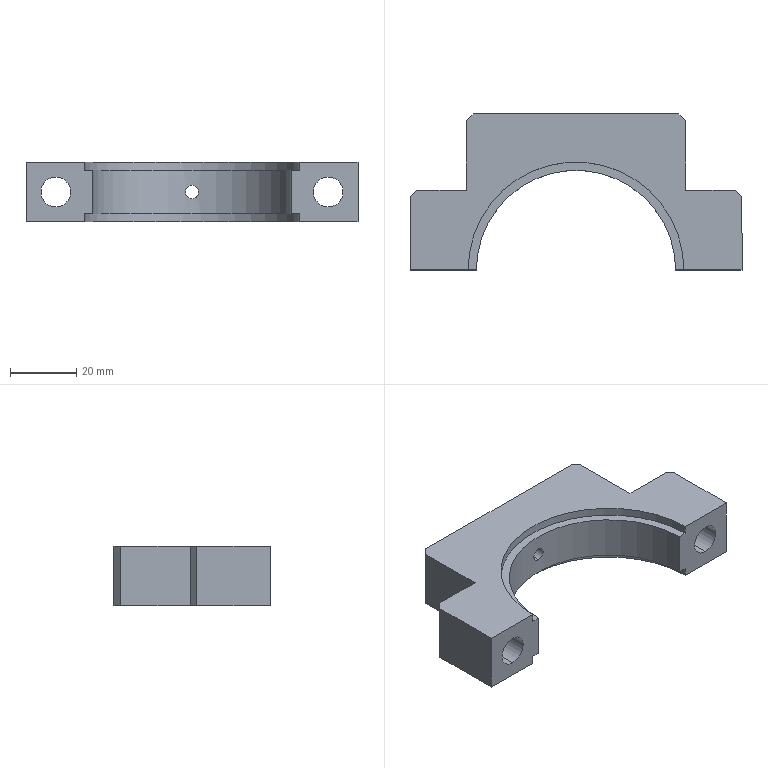Part | SolidWorks | features HoleWzd 3, ICE 2, Chamfer 1, Extrusion 1 | 1 solid | 30 faces | box 100 x 47 x 18 mm | volume 40091 mm3 | plane 17 | cylinder 11 | cone 2 | commonest cylinder face diameters 9 x4 4 x2 7 x2 65 x2 60 x1
STEP:
#1=CARTESIAN_POINT('',(0.,30.,7.));
#2=VERTEX_POINT('',#1);
#3=CARTESIAN_POINT('',(0.,30.,11.));
#4=VERTEX_POINT('',#3);
#5=CARTESIAN_POINT('',(0.,30.,7.));
#6=CARTESIAN_POINT('',(-0.261,30.,7.));
#7=CARTESIAN_POINT('',(-0.5242,29.996,7.052));
#8=CARTESIAN_POINT('',(-1.006,29.984,7.252));
#9=CARTESIAN_POINT('',(-1.229,29.975,7.401));
#10=CARTESIAN_POINT('',(-1.505,29.962,7.677));
#11=CARTESIAN_POINT('',(-1.59,29.958,7.78));
#12=CARTESIAN_POINT('',(-1.735,29.95,7.997));
#13=CARTESIAN_POINT('',(-1.797,29.946,8.112));
#14=CARTESIAN_POINT('',(-1.897,29.94,8.354));
#15=CARTESIAN_POINT('',(-1.936,29.937,8.481));
#16=CARTESIAN_POINT('',(-1.987,29.934,8.737));
#17=CARTESIAN_POINT('',(-2.,29.933,8.866));
#18=CARTESIAN_POINT('',(-2.,29.933,9.13));
#19=CARTESIAN_POINT('',(-1.987,29.934,9.261));
#20=CARTESIAN_POINT('',(-1.937,29.937,9.516));
#21=CARTESIAN_POINT('',(-1.898,29.94,9.643));
#22=CARTESIAN_POINT('',(-1.798,29.946,9.886));
#23=CARTESIAN_POINT('',(-1.737,29.95,10.001));
#24=CARTESIAN_POINT('',(-1.592,29.958,10.218));
#25=CARTESIAN_POINT('',(-1.507,29.962,10.321));
#26=CARTESIAN_POINT('',(-1.323,29.971,10.506));
#27=CARTESIAN_POINT('',(-1.222,29.975,10.588));
#28=CARTESIAN_POINT('',(-1.004,29.983,10.735));
#29=CARTESIAN_POINT('',(-0.8877,29.987,10.797));
#30=CARTESIAN_POINT('',(-0.5269,29.996,10.947));
#31=CARTESIAN_POINT('',(-0.2643,30.,11.));
#32=CARTESIAN_POINT('',(0.,30.,11.));
#33=B_SPLINE_CURVE_WITH_KNOTS('',3,(#5,#6,#7,#8,#9,#10,#11,#12,#13,#14,#15,#16,#17,#18,#19,#20,#21,#22,#23,#24,#25,#26,#27,#28,#29,#30,#31,#32),.UNSPECIFIED.,.F.,.F.,(4,2,2,2,2,2,2,2,2,2,2,2,2,4),(0.006255,0.007036,0.007818,0.008209,0.0086,0.00899,0.009381,0.009772,0.01016,0.01055,0.01094,0.01134,0.01173,0.01251),.UNSPECIFIED.);
#34=EDGE_CURVE('',#2,#4,#33,.T.);
#35=ORIENTED_EDGE('',*,*,#34,.F.);
#36=CARTESIAN_POINT('',(0.,33.099,7.));
#37=VERTEX_POINT('',#36);
#38=CARTESIAN_POINT('',(0.,47.,7.));
#39=DIRECTION('',(0.,1.,0.));
#40=VECTOR('',#39,1000.);
#41=LINE('',#38,#40);
#42=EDGE_CURVE('',#2,#37,#41,.T.);
#43=ORIENTED_EDGE('',*,*,#42,.T.);
#44=CARTESIAN_POINT('',(0.,33.099,11.));
#45=VERTEX_POINT('',#44);
#46=CARTESIAN_POINT('',(0.,33.099,9.));
#47=DIRECTION('',(0.,-1.,0.));
#48=DIRECTION('',(0.,0.,1.));
#49=AXIS2_PLACEMENT_3D('',#46,#47,#48);
#50=CIRCLE('',#49,2.);
#51=EDGE_CURVE('',#45,#37,#50,.T.);
#52=ORIENTED_EDGE('',*,*,#51,.F.);
#53=CARTESIAN_POINT('',(0.,47.,11.));
#54=DIRECTION('',(0.,1.,0.));
#55=VECTOR('',#54,1000.);
#56=LINE('',#53,#55);
#57=EDGE_CURVE('',#4,#45,#56,.T.);
#58=ORIENTED_EDGE('',*,*,#57,.F.);
#59=EDGE_LOOP('',(#35,#43,#52,#58));
#60=FACE_OUTER_BOUND('',#59,.T.);
#61=CARTESIAN_POINT('',(0.,47.,9.));
#62=DIRECTION('',(0.,1.,0.));
#63=DIRECTION('',(0.,0.,1.));
#64=AXIS2_PLACEMENT_3D('',#61,#62,#63);
#65=CYLINDRICAL_SURFACE('',#64,2.);
#66=ADVANCED_FACE('',(#60),#65,.F.);
#67=CARTESIAN_POINT('',(-41.,0.,4.5));
#68=VERTEX_POINT('',#67);
#69=CARTESIAN_POINT('',(-41.,0.,13.5));
#70=VERTEX_POINT('',#69);
#71=CARTESIAN_POINT('',(-41.,0.,9.));
#72=DIRECTION('',(0.,1.,0.));
#73=DIRECTION('',(0.,0.,1.));
#74=AXIS2_PLACEMENT_3D('',#71,#72,#73);
#75=CIRCLE('',#74,4.5);
#76=EDGE_CURVE('',#68,#70,#75,.T.);
#77=ORIENTED_EDGE('',*,*,#76,.F.);
#78=CARTESIAN_POINT('',(-41.,24.,4.5));
#79=VERTEX_POINT('',#78);
#80=CARTESIAN_POINT('',(-41.,24.,4.5));
#81=DIRECTION('',(0.,1.,0.));
#82=VECTOR('',#81,1000.);
#83=LINE('',#80,#82);
#84=EDGE_CURVE('',#68,#79,#83,.T.);
#85=ORIENTED_EDGE('',*,*,#84,.T.);
#86=CARTESIAN_POINT('',(-41.,24.,13.5));
#87=VERTEX_POINT('',#86);
#88=CARTESIAN_POINT('',(-41.,24.,9.));
#89=DIRECTION('',(0.,1.,0.));
#90=DIRECTION('',(0.,0.,1.));
#91=AXIS2_PLACEMENT_3D('',#88,#89,#90);
#92=CIRCLE('',#91,4.5);
#93=EDGE_CURVE('',#79,#87,#92,.T.);
#94=ORIENTED_EDGE('',*,*,#93,.T.);
#95=CARTESIAN_POINT('',(-41.,24.,13.5));
#96=DIRECTION('',(0.,1.,0.));
#97=VECTOR('',#96,1000.);
#98=LINE('',#95,#97);
#99=EDGE_CURVE('',#70,#87,#98,.T.);
#100=ORIENTED_EDGE('',*,*,#99,.F.);
#101=EDGE_LOOP('',(#77,#85,#94,#100));
#102=FACE_OUTER_BOUND('',#101,.T.);
#103=CARTESIAN_POINT('',(-41.,24.,9.));
#104=DIRECTION('',(0.,1.,0.));
#105=DIRECTION('',(0.,0.,1.));
#106=AXIS2_PLACEMENT_3D('',#103,#104,#105);
#107=CYLINDRICAL_SURFACE('',#106,4.5);
#108=ADVANCED_FACE('',(#102),#107,.F.);
#109=CARTESIAN_POINT('',(41.,0.,4.5));
#110=VERTEX_POINT('',#109);
#111=CARTESIAN_POINT('',(41.,0.,13.5));
#112=VERTEX_POINT('',#111);
#113=CARTESIAN_POINT('',(41.,0.,9.));
#114=DIRECTION('',(0.,1.,0.));
#115=DIRECTION('',(0.,0.,1.));
#116=AXIS2_PLACEMENT_3D('',#113,#114,#115);
#117=CIRCLE('',#116,4.5);
#118=EDGE_CURVE('',#110,#112,#117,.T.);
#119=ORIENTED_EDGE('',*,*,#118,.F.);
#120=CARTESIAN_POINT('',(41.,24.,4.5));
#121=VERTEX_POINT('',#120);
#122=CARTESIAN_POINT('',(41.,24.,4.5));
#123=DIRECTION('',(0.,1.,0.));
#124=VECTOR('',#123,1000.);
#125=LINE('',#122,#124);
#126=EDGE_CURVE('',#110,#121,#125,.T.);
#127=ORIENTED_EDGE('',*,*,#126,.T.);
#128=CARTESIAN_POINT('',(41.,24.,13.5));
#129=VERTEX_POINT('',#128);
#130=CARTESIAN_POINT('',(41.,24.,9.));
#131=DIRECTION('',(0.,1.,0.));
#132=DIRECTION('',(0.,0.,1.));
#133=AXIS2_PLACEMENT_3D('',#130,#131,#132);
#134=CIRCLE('',#133,4.5);
#135=EDGE_CURVE('',#121,#129,#134,.T.);
#136=ORIENTED_EDGE('',*,*,#135,.T.);
#137=CARTESIAN_POINT('',(41.,24.,13.5));
#138=DIRECTION('',(0.,1.,0.));
#139=VECTOR('',#138,1000.);
#140=LINE('',#137,#139);
#141=EDGE_CURVE('',#112,#129,#140,.T.);
#142=ORIENTED_EDGE('',*,*,#141,.F.);
#143=EDGE_LOOP('',(#119,#127,#136,#142));
#144=FACE_OUTER_BOUND('',#143,.T.);
#145=CARTESIAN_POINT('',(41.,24.,9.));
#146=DIRECTION('',(0.,1.,0.));
#147=DIRECTION('',(0.,0.,1.));
#148=AXIS2_PLACEMENT_3D('',#145,#146,#147);
#149=CYLINDRICAL_SURFACE('',#148,4.5);
#150=ADVANCED_FACE('',(#144),#149,.F.);
#151=CARTESIAN_POINT('',(0.,34.,5.5));
#152=VERTEX_POINT('',#151);
#153=CARTESIAN_POINT('',(0.,34.,12.5));
#154=VERTEX_POINT('',#153);
#155=CARTESIAN_POINT('',(0.,34.,9.));
#156=DIRECTION('',(0.,1.,0.));
#157=DIRECTION('',(0.,0.,1.));
#158=AXIS2_PLACEMENT_3D('',#155,#156,#157);
#159=CIRCLE('',#158,3.5);
#160=EDGE_CURVE('',#152,#154,#159,.T.);
#161=ORIENTED_EDGE('',*,*,#160,.F.);
#162=CARTESIAN_POINT('',(0.,47.,5.5));
#163=VERTEX_POINT('',#162);
#164=CARTESIAN_POINT('',(0.,47.,5.5));
#165=DIRECTION('',(0.,1.,0.));
#166=VECTOR('',#165,1000.);
#167=LINE('',#164,#166);
#168=EDGE_CURVE('',#152,#163,#167,.T.);
#169=ORIENTED_EDGE('',*,*,#168,.T.);
#170=CARTESIAN_POINT('',(0.,47.,12.5));
#171=VERTEX_POINT('',#170);
#172=CARTESIAN_POINT('',(0.,47.,9.));
#173=DIRECTION('',(0.,1.,0.));
#174=DIRECTION('',(0.,0.,1.));
#175=AXIS2_PLACEMENT_3D('',#172,#173,#174);
#176=CIRCLE('',#175,3.5);
#177=EDGE_CURVE('',#163,#171,#176,.T.);
#178=ORIENTED_EDGE('',*,*,#177,.T.);
#179=CARTESIAN_POINT('',(0.,47.,12.5));
#180=DIRECTION('',(0.,1.,0.));
#181=VECTOR('',#180,1000.);
#182=LINE('',#179,#181);
#183=EDGE_CURVE('',#154,#171,#182,.T.);
#184=ORIENTED_EDGE('',*,*,#183,.F.);
#185=EDGE_LOOP('',(#161,#169,#178,#184));
#186=FACE_OUTER_BOUND('',#185,.T.);
#187=CARTESIAN_POINT('',(0.,47.,9.));
#188=DIRECTION('',(0.,1.,0.));
#189=DIRECTION('',(0.,0.,1.));
#190=AXIS2_PLACEMENT_3D('',#187,#188,#189);
#191=CYLINDRICAL_SURFACE('',#190,3.5);
#192=ADVANCED_FACE('',(#186),#191,.F.);
#193=ORIENTED_EDGE('',*,*,#51,.T.);
#194=CARTESIAN_POINT('',(0.,34.,5.5));
#195=DIRECTION('',(0.,0.515,-0.8572));
#196=VECTOR('',#195,1000.);
#197=LINE('',#194,#196);
#198=EDGE_CURVE('',#37,#152,#197,.T.);
#199=ORIENTED_EDGE('',*,*,#198,.T.);
#200=ORIENTED_EDGE('',*,*,#160,.T.);
#201=CARTESIAN_POINT('',(0.,34.,12.5));
#202=DIRECTION('',(0.,0.515,0.8572));
#203=VECTOR('',#202,1000.);
#204=LINE('',#201,#203);
#205=EDGE_CURVE('',#45,#154,#204,.T.);
#206=ORIENTED_EDGE('',*,*,#205,.F.);
#207=EDGE_LOOP('',(#193,#199,#200,#206));
#208=FACE_OUTER_BOUND('',#207,.T.);
#209=CARTESIAN_POINT('',(0.,34.,9.));
#210=DIRECTION('',(0.,1.,0.));
#211=DIRECTION('',(0.,0.,1.));
#212=AXIS2_PLACEMENT_3D('',#209,#210,#211);
#213=CONICAL_SURFACE('',#212,3.5,1.03);
#214=ADVANCED_FACE('',(#208),#213,.F.);
#215=CARTESIAN_POINT('',(0.,30.,11.));
#216=CARTESIAN_POINT('',(0.1322,30.,11.));
#217=CARTESIAN_POINT('',(0.2622,29.999,10.987));
#218=CARTESIAN_POINT('',(0.5178,29.996,10.936));
#219=CARTESIAN_POINT('',(0.6449,29.993,10.898));
#220=CARTESIAN_POINT('',(0.8871,29.987,10.797));
#221=CARTESIAN_POINT('',(1.002,29.983,10.736));
#222=CARTESIAN_POINT('',(1.219,29.975,10.591));
#223=CARTESIAN_POINT('',(1.322,29.971,10.506));
#224=CARTESIAN_POINT('',(1.599,29.958,10.229));
#225=CARTESIAN_POINT('',(1.748,29.949,10.006));
#226=CARTESIAN_POINT('',(1.947,29.937,9.525));
#227=CARTESIAN_POINT('',(2.,29.933,9.262));
#228=CARTESIAN_POINT('',(2.,29.933,8.87));
#229=CARTESIAN_POINT('',(1.987,29.934,8.738));
#230=CARTESIAN_POINT('',(1.936,29.937,8.481));
#231=CARTESIAN_POINT('',(1.898,29.94,8.356));
#232=CARTESIAN_POINT('',(1.798,29.946,8.114));
#233=CARTESIAN_POINT('',(1.735,29.95,7.997));
#234=CARTESIAN_POINT('',(1.591,29.958,7.78));
#235=CARTESIAN_POINT('',(1.508,29.962,7.679));
#236=CARTESIAN_POINT('',(1.321,29.971,7.493));
#237=CARTESIAN_POINT('',(1.22,29.975,7.41));
#238=CARTESIAN_POINT('',(1.003,29.983,7.265));
#239=CARTESIAN_POINT('',(0.8865,29.987,7.202));
#240=CARTESIAN_POINT('',(0.6442,29.993,7.102));
#241=CARTESIAN_POINT('',(0.5195,29.996,7.064));
#242=CARTESIAN_POINT('',(0.2631,29.999,7.013));
#243=CARTESIAN_POINT('',(0.1305,30.,7.));
#244=CARTESIAN_POINT('',(0.,30.,7.));
#245=B_SPLINE_CURVE_WITH_KNOTS('',3,(#215,#216,#217,#218,#219,#220,#221,#222,#223,#224,#225,#226,#227,#228,#229,#230,#231,#232,#233,#234,#235,#236,#237,#238,#239,#240,#241,#242,#243,#244),.UNSPECIFIED.,.F.,.F.,(4,2,2,2,2,2,2,2,2,2,2,2,2,2,4),(0.,0.0003909,0.0007818,0.001173,0.001564,0.002345,0.003127,0.003518,0.003909,0.0043,0.004691,0.005082,0.005473,0.005864,0.006255),.UNSPECIFIED.);
#246=EDGE_CURVE('',#4,#2,#245,.T.);
#247=ORIENTED_EDGE('',*,*,#246,.T.);
#248=ORIENTED_EDGE('',*,*,#34,.T.);
#249=EDGE_LOOP('',(#247,#248));
#250=FACE_BOUND('',#249,.T.);
#251=CARTESIAN_POINT('',(-30.,0.,15.5));
#252=VERTEX_POINT('',#251);
#253=CARTESIAN_POINT('',(30.,0.,15.5));
#254=VERTEX_POINT('',#253);
#255=CARTESIAN_POINT('',(0.,0.,15.5));
#256=DIRECTION('',(0.,0.,-1.));
#257=DIRECTION('',(1.,0.,0.));
#258=AXIS2_PLACEMENT_3D('',#255,#256,#257);
#259=CIRCLE('',#258,30.);
#260=EDGE_CURVE('',#252,#254,#259,.T.);
#261=ORIENTED_EDGE('',*,*,#260,.F.);
#262=CARTESIAN_POINT('',(-30.,0.,2.5));
#263=VERTEX_POINT('',#262);
#264=CARTESIAN_POINT('',(-30.,0.,18.));
#265=DIRECTION('',(0.,0.,-1.));
#266=VECTOR('',#265,1000.);
#267=LINE('',#264,#266);
#268=EDGE_CURVE('',#252,#263,#267,.T.);
#269=ORIENTED_EDGE('',*,*,#268,.T.);
#270=CARTESIAN_POINT('',(30.,0.,2.5));
#271=VERTEX_POINT('',#270);
#272=CARTESIAN_POINT('',(0.,0.,2.5));
#273=DIRECTION('',(0.,0.,1.));
#274=DIRECTION('',(-1.,0.,0.));
#275=AXIS2_PLACEMENT_3D('',#272,#273,#274);
#276=CIRCLE('',#275,30.);
#277=EDGE_CURVE('',#271,#263,#276,.T.);
#278=ORIENTED_EDGE('',*,*,#277,.F.);
#279=CARTESIAN_POINT('',(30.,0.,18.));
#280=DIRECTION('',(0.,0.,-1.));
#281=VECTOR('',#280,1000.);
#282=LINE('',#279,#281);
#283=EDGE_CURVE('',#254,#271,#282,.T.);
#284=ORIENTED_EDGE('',*,*,#283,.F.);
#285=EDGE_LOOP('',(#261,#269,#278,#284));
#286=FACE_OUTER_BOUND('',#285,.T.);
#287=CARTESIAN_POINT('',(0.,0.,18.));
#288=DIRECTION('',(0.,0.,-1.));
#289=DIRECTION('',(-1.,0.,0.));
#290=AXIS2_PLACEMENT_3D('',#287,#288,#289);
#291=CYLINDRICAL_SURFACE('',#290,30.);
#292=ADVANCED_FACE('',(#250,#286),#291,.F.);
#293=CARTESIAN_POINT('',(-50.,22.,18.));
#294=VERTEX_POINT('',#293);
#295=CARTESIAN_POINT('',(-50.,0.,18.));
#296=VERTEX_POINT('',#295);
#297=CARTESIAN_POINT('',(-50.,0.,18.));
#298=DIRECTION('',(0.,-1.,0.));
#299=VECTOR('',#298,1000.);
#300=LINE('',#297,#299);
#301=EDGE_CURVE('',#294,#296,#300,.T.);
#302=ORIENTED_EDGE('',*,*,#301,.F.);
#303=CARTESIAN_POINT('',(-50.,22.,0.));
#304=VERTEX_POINT('',#303);
#305=CARTESIAN_POINT('',(-50.,22.,18.));
#306=DIRECTION('',(0.,0.,-1.));
#307=VECTOR('',#306,1000.);
#308=LINE('',#305,#307);
#309=EDGE_CURVE('',#294,#304,#308,.T.);
#310=ORIENTED_EDGE('',*,*,#309,.T.);
#311=CARTESIAN_POINT('',(-50.,0.,0.));
#312=VERTEX_POINT('',#311);
#313=CARTESIAN_POINT('',(-50.,0.,0.));
#314=DIRECTION('',(0.,-1.,0.));
#315=VECTOR('',#314,1000.);
#316=LINE('',#313,#315);
#317=EDGE_CURVE('',#304,#312,#316,.T.);
#318=ORIENTED_EDGE('',*,*,#317,.T.);
#319=CARTESIAN_POINT('',(-50.,0.,18.));
#320=DIRECTION('',(0.,0.,-1.));
#321=VECTOR('',#320,1000.);
#322=LINE('',#319,#321);
#323=EDGE_CURVE('',#296,#312,#322,.T.);
#324=ORIENTED_EDGE('',*,*,#323,.F.);
#325=EDGE_LOOP('',(#302,#310,#318,#324));
#326=FACE_OUTER_BOUND('',#325,.T.);
#327=CARTESIAN_POINT('',(-50.,0.,18.));
#328=DIRECTION('',(1.,0.,0.));
#329=DIRECTION('',(0.,0.,-1.));
#330=AXIS2_PLACEMENT_3D('',#327,#328,#329);
#331=PLANE('',#330);
#332=ADVANCED_FACE('',(#326),#331,.F.);
#333=CARTESIAN_POINT('',(-41.,0.,9.));
#334=DIRECTION('',(0.,1.,0.));
#335=DIRECTION('',(0.,0.,1.));
#336=AXIS2_PLACEMENT_3D('',#333,#334,#335);
#337=CIRCLE('',#336,4.5);
#338=EDGE_CURVE('',#70,#68,#337,.T.);
#339=ORIENTED_EDGE('',*,*,#338,.T.);
#340=ORIENTED_EDGE('',*,*,#76,.T.);
#341=EDGE_LOOP('',(#339,#340));
#342=FACE_BOUND('',#341,.T.);
#343=CARTESIAN_POINT('',(-32.5,0.,15.5));
#344=VERTEX_POINT('',#343);
#345=CARTESIAN_POINT('',(-50.,0.,15.5));
#346=DIRECTION('',(1.,0.,0.));
#347=VECTOR('',#346,1000.);
#348=LINE('',#345,#347);
#349=EDGE_CURVE('',#344,#252,#348,.T.);
#350=ORIENTED_EDGE('',*,*,#349,.F.);
#351=CARTESIAN_POINT('',(-32.5,0.,18.));
#352=VERTEX_POINT('',#351);
#353=CARTESIAN_POINT('',(-32.5,0.,15.5));
#354=DIRECTION('',(0.,0.,1.));
#355=VECTOR('',#354,1000.);
#356=LINE('',#353,#355);
#357=EDGE_CURVE('',#344,#352,#356,.T.);
#358=ORIENTED_EDGE('',*,*,#357,.T.);
#359=CARTESIAN_POINT('',(-50.,0.,18.));
#360=DIRECTION('',(1.,0.,0.));
#361=VECTOR('',#360,1000.);
#362=LINE('',#359,#361);
#363=EDGE_CURVE('',#296,#352,#362,.T.);
#364=ORIENTED_EDGE('',*,*,#363,.F.);
#365=ORIENTED_EDGE('',*,*,#323,.T.);
#366=CARTESIAN_POINT('',(-32.5,0.,0.));
#367=VERTEX_POINT('',#366);
#368=CARTESIAN_POINT('',(-50.,0.,0.));
#369=DIRECTION('',(1.,0.,0.));
#370=VECTOR('',#369,1000.);
#371=LINE('',#368,#370);
#372=EDGE_CURVE('',#312,#367,#371,.T.);
#373=ORIENTED_EDGE('',*,*,#372,.T.);
#374=CARTESIAN_POINT('',(-32.5,0.,2.5));
#375=VERTEX_POINT('',#374);
#376=CARTESIAN_POINT('',(-32.5,0.,2.5));
#377=DIRECTION('',(0.,0.,1.));
#378=VECTOR('',#377,1000.);
#379=LINE('',#376,#378);
#380=EDGE_CURVE('',#367,#375,#379,.T.);
#381=ORIENTED_EDGE('',*,*,#380,.T.);
#382=CARTESIAN_POINT('',(-50.,0.,2.5));
#383=DIRECTION('',(-1.,0.,0.));
#384=VECTOR('',#383,1000.);
#385=LINE('',#382,#384);
#386=EDGE_CURVE('',#263,#375,#385,.T.);
#387=ORIENTED_EDGE('',*,*,#386,.F.);
#388=ORIENTED_EDGE('',*,*,#268,.F.);
#389=EDGE_LOOP('',(#350,#358,#364,#365,#373,#381,#387,#388));
#390=FACE_OUTER_BOUND('',#389,.T.);
#391=CARTESIAN_POINT('',(-50.,0.,18.));
#392=DIRECTION('',(0.,1.,0.));
#393=DIRECTION('',(-1.,0.,0.));
#394=AXIS2_PLACEMENT_3D('',#391,#392,#393);
#395=PLANE('',#394);
#396=ADVANCED_FACE('',(#342,#390),#395,.F.);
#397=CARTESIAN_POINT('',(41.,0.,9.));
#398=DIRECTION('',(0.,1.,0.));
#399=DIRECTION('',(0.,0.,1.));
#400=AXIS2_PLACEMENT_3D('',#397,#398,#399);
#401=CIRCLE('',#400,4.5);
#402=EDGE_CURVE('',#112,#110,#401,.T.);
#403=ORIENTED_EDGE('',*,*,#402,.T.);
#404=ORIENTED_EDGE('',*,*,#118,.T.);
#405=EDGE_LOOP('',(#403,#404));
#406=FACE_BOUND('',#405,.T.);
#407=CARTESIAN_POINT('',(32.5,0.,18.));
#408=VERTEX_POINT('',#407);
#409=CARTESIAN_POINT('',(50.,0.,18.));
#410=VERTEX_POINT('',#409);
#411=CARTESIAN_POINT('',(30.,0.,18.));
#412=DIRECTION('',(1.,0.,0.));
#413=VECTOR('',#412,1000.);
#414=LINE('',#411,#413);
#415=EDGE_CURVE('',#408,#410,#414,.T.);
#416=ORIENTED_EDGE('',*,*,#415,.F.);
#417=CARTESIAN_POINT('',(32.5,0.,15.5));
#418=VERTEX_POINT('',#417);
#419=CARTESIAN_POINT('',(32.5,0.,15.5));
#420=DIRECTION('',(0.,0.,-1.));
#421=VECTOR('',#420,1000.);
#422=LINE('',#419,#421);
#423=EDGE_CURVE('',#408,#418,#422,.T.);
#424=ORIENTED_EDGE('',*,*,#423,.T.);
#425=CARTESIAN_POINT('',(30.,0.,15.5));
#426=DIRECTION('',(1.,0.,0.));
#427=VECTOR('',#426,1000.);
#428=LINE('',#425,#427);
#429=EDGE_CURVE('',#254,#418,#428,.T.);
#430=ORIENTED_EDGE('',*,*,#429,.F.);
#431=ORIENTED_EDGE('',*,*,#283,.T.);
#432=CARTESIAN_POINT('',(32.5,0.,2.5));
#433=VERTEX_POINT('',#432);
#434=CARTESIAN_POINT('',(30.,0.,2.5));
#435=DIRECTION('',(-1.,0.,0.));
#436=VECTOR('',#435,1000.);
#437=LINE('',#434,#436);
#438=EDGE_CURVE('',#433,#271,#437,.T.);
#439=ORIENTED_EDGE('',*,*,#438,.F.);
#440=CARTESIAN_POINT('',(32.5,0.,0.));
#441=VERTEX_POINT('',#440);
#442=CARTESIAN_POINT('',(32.5,0.,2.5));
#443=DIRECTION('',(0.,0.,-1.));
#444=VECTOR('',#443,1000.);
#445=LINE('',#442,#444);
#446=EDGE_CURVE('',#433,#441,#445,.T.);
#447=ORIENTED_EDGE('',*,*,#446,.T.);
#448=CARTESIAN_POINT('',(50.,0.,0.));
#449=VERTEX_POINT('',#448);
#450=CARTESIAN_POINT('',(30.,0.,0.));
#451=DIRECTION('',(1.,0.,0.));
#452=VECTOR('',#451,1000.);
#453=LINE('',#450,#452);
#454=EDGE_CURVE('',#441,#449,#453,.T.);
#455=ORIENTED_EDGE('',*,*,#454,.T.);
#456=CARTESIAN_POINT('',(50.,0.,18.));
#457=DIRECTION('',(0.,0.,-1.));
#458=VECTOR('',#457,1000.);
#459=LINE('',#456,#458);
#460=EDGE_CURVE('',#410,#449,#459,.T.);
#461=ORIENTED_EDGE('',*,*,#460,.F.);
#462=EDGE_LOOP('',(#416,#424,#430,#431,#439,#447,#455,#461));
#463=FACE_OUTER_BOUND('',#462,.T.);
#464=CARTESIAN_POINT('',(30.,0.,18.));
#465=DIRECTION('',(0.,1.,0.));
#466=DIRECTION('',(-1.,0.,0.));
#467=AXIS2_PLACEMENT_3D('',#464,#465,#466);
#468=PLANE('',#467);
#469=ADVANCED_FACE('',(#406,#463),#468,.F.);
#470=CARTESIAN_POINT('',(50.,22.,0.));
#471=VERTEX_POINT('',#470);
#472=CARTESIAN_POINT('',(50.,0.,0.));
#473=DIRECTION('',(0.,1.,0.));
#474=VECTOR('',#473,1000.);
#475=LINE('',#472,#474);
#476=EDGE_CURVE('',#449,#471,#475,.T.);
#477=ORIENTED_EDGE('',*,*,#476,.T.);
#478=CARTESIAN_POINT('',(50.,22.,18.));
#479=VERTEX_POINT('',#478);
#480=CARTESIAN_POINT('',(50.,22.,18.));
#481=DIRECTION('',(0.,0.,1.));
#482=VECTOR('',#481,1000.);
#483=LINE('',#480,#482);
#484=EDGE_CURVE('',#471,#479,#483,.T.);
#485=ORIENTED_EDGE('',*,*,#484,.T.);
#486=CARTESIAN_POINT('',(50.,0.,18.));
#487=DIRECTION('',(0.,1.,0.));
#488=VECTOR('',#487,1000.);
#489=LINE('',#486,#488);
#490=EDGE_CURVE('',#410,#479,#489,.T.);
#491=ORIENTED_EDGE('',*,*,#490,.F.);
#492=ORIENTED_EDGE('',*,*,#460,.T.);
#493=EDGE_LOOP('',(#477,#485,#491,#492));
#494=FACE_OUTER_BOUND('',#493,.T.);
#495=CARTESIAN_POINT('',(50.,0.,18.));
#496=DIRECTION('',(-1.,0.,0.));
#497=DIRECTION('',(0.,-1.,0.));
#498=AXIS2_PLACEMENT_3D('',#495,#496,#497);
#499=PLANE('',#498);
#500=ADVANCED_FACE('',(#494),#499,.F.);
#501=CARTESIAN_POINT('',(41.,24.,9.));
#502=DIRECTION('',(0.,1.,0.));
#503=DIRECTION('',(0.,0.,1.));
#504=AXIS2_PLACEMENT_3D('',#501,#502,#503);
#505=CIRCLE('',#504,4.5);
#506=EDGE_CURVE('',#129,#121,#505,.T.);
#507=ORIENTED_EDGE('',*,*,#506,.F.);
#508=ORIENTED_EDGE('',*,*,#135,.F.);
#509=EDGE_LOOP('',(#507,#508));
#510=FACE_BOUND('',#509,.T.);
#511=CARTESIAN_POINT('',(48.,24.,18.));
#512=VERTEX_POINT('',#511);
#513=CARTESIAN_POINT('',(33.,24.,18.));
#514=VERTEX_POINT('',#513);
#515=CARTESIAN_POINT('',(50.,24.,18.));
#516=DIRECTION('',(-1.,0.,0.));
#517=VECTOR('',#516,1000.);
#518=LINE('',#515,#517);
#519=EDGE_CURVE('',#512,#514,#518,.T.);
#520=ORIENTED_EDGE('',*,*,#519,.F.);
#521=CARTESIAN_POINT('',(48.,24.,0.));
#522=VERTEX_POINT('',#521);
#523=CARTESIAN_POINT('',(48.,24.,18.));
#524=DIRECTION('',(0.,0.,-1.));
#525=VECTOR('',#524,1000.);
#526=LINE('',#523,#525);
#527=EDGE_CURVE('',#512,#522,#526,.T.);
#528=ORIENTED_EDGE('',*,*,#527,.T.);
#529=CARTESIAN_POINT('',(33.,24.,0.));
#530=VERTEX_POINT('',#529);
#531=CARTESIAN_POINT('',(50.,24.,0.));
#532=DIRECTION('',(-1.,0.,0.));
#533=VECTOR('',#532,1000.);
#534=LINE('',#531,#533);
#535=EDGE_CURVE('',#522,#530,#534,.T.);
#536=ORIENTED_EDGE('',*,*,#535,.T.);
#537=CARTESIAN_POINT('',(33.,24.,18.));
#538=DIRECTION('',(0.,0.,-1.));
#539=VECTOR('',#538,1000.);
#540=LINE('',#537,#539);
#541=EDGE_CURVE('',#514,#530,#540,.T.);
#542=ORIENTED_EDGE('',*,*,#541,.F.);
#543=EDGE_LOOP('',(#520,#528,#536,#542));
#544=FACE_OUTER_BOUND('',#543,.T.);
#545=CARTESIAN_POINT('',(50.,24.,18.));
#546=DIRECTION('',(0.,-1.,0.));
#547=DIRECTION('',(1.,0.,0.));
#548=AXIS2_PLACEMENT_3D('',#545,#546,#547);
#549=PLANE('',#548);
#550=ADVANCED_FACE('',(#510,#544),#549,.F.);
#551=CARTESIAN_POINT('',(33.,45.,0.));
#552=VERTEX_POINT('',#551);
#553=CARTESIAN_POINT('',(33.,24.,0.));
#554=DIRECTION('',(0.,1.,0.));
#555=VECTOR('',#554,1000.);
#556=LINE('',#553,#555);
#557=EDGE_CURVE('',#530,#552,#556,.T.);
#558=ORIENTED_EDGE('',*,*,#557,.T.);
#559=CARTESIAN_POINT('',(33.,45.,18.));
#560=VERTEX_POINT('',#559);
#561=CARTESIAN_POINT('',(33.,45.,18.));
#562=DIRECTION('',(0.,0.,1.));
#563=VECTOR('',#562,1000.);
#564=LINE('',#561,#563);
#565=EDGE_CURVE('',#552,#560,#564,.T.);
#566=ORIENTED_EDGE('',*,*,#565,.T.);
#567=CARTESIAN_POINT('',(33.,24.,18.));
#568=DIRECTION('',(0.,1.,0.));
#569=VECTOR('',#568,1000.);
#570=LINE('',#567,#569);
#571=EDGE_CURVE('',#514,#560,#570,.T.);
#572=ORIENTED_EDGE('',*,*,#571,.F.);
#573=ORIENTED_EDGE('',*,*,#541,.T.);
#574=EDGE_LOOP('',(#558,#566,#572,#573));
#575=FACE_OUTER_BOUND('',#574,.T.);
#576=CARTESIAN_POINT('',(33.,24.,18.));
#577=DIRECTION('',(-1.,0.,0.));
#578=DIRECTION('',(0.,-1.,0.));
#579=AXIS2_PLACEMENT_3D('',#576,#577,#578);
#580=PLANE('',#579);
#581=ADVANCED_FACE('',(#575),#580,.F.);
#582=CARTESIAN_POINT('',(0.,47.,9.));
#583=DIRECTION('',(0.,1.,0.));
#584=DIRECTION('',(0.,0.,1.));
#585=AXIS2_PLACEMENT_3D('',#582,#583,#584);
#586=CIRCLE('',#585,3.5);
#587=EDGE_CURVE('',#171,#163,#586,.T.);
#588=ORIENTED_EDGE('',*,*,#587,.F.);
#589=ORIENTED_EDGE('',*,*,#177,.F.);
#590=EDGE_LOOP('',(#588,#589));
#591=FACE_BOUND('',#590,.T.);
#592=CARTESIAN_POINT('',(31.,47.,18.));
#593=VERTEX_POINT('',#592);
#594=CARTESIAN_POINT('',(-31.,47.,18.));
#595=VERTEX_POINT('',#594);
#596=CARTESIAN_POINT('',(-33.,47.,18.));
#597=DIRECTION('',(-1.,0.,0.));
#598=VECTOR('',#597,1000.);
#599=LINE('',#596,#598);
#600=EDGE_CURVE('',#593,#595,#599,.T.);
#601=ORIENTED_EDGE('',*,*,#600,.F.);
#602=CARTESIAN_POINT('',(31.,47.,0.));
#603=VERTEX_POINT('',#602);
#604=CARTESIAN_POINT('',(31.,47.,18.));
#605=DIRECTION('',(0.,0.,-1.));
#606=VECTOR('',#605,1000.);
#607=LINE('',#604,#606);
#608=EDGE_CURVE('',#593,#603,#607,.T.);
#609=ORIENTED_EDGE('',*,*,#608,.T.);
#610=CARTESIAN_POINT('',(-31.,47.,0.));
#611=VERTEX_POINT('',#610);
#612=CARTESIAN_POINT('',(-33.,47.,0.));
#613=DIRECTION('',(-1.,0.,0.));
#614=VECTOR('',#613,1000.);
#615=LINE('',#612,#614);
#616=EDGE_CURVE('',#603,#611,#615,.T.);
#617=ORIENTED_EDGE('',*,*,#616,.T.);
#618=CARTESIAN_POINT('',(-31.,47.,18.));
#619=DIRECTION('',(0.,0.,1.));
#620=VECTOR('',#619,1000.);
#621=LINE('',#618,#620);
#622=EDGE_CURVE('',#611,#595,#621,.T.);
#623=ORIENTED_EDGE('',*,*,#622,.T.);
#624=EDGE_LOOP('',(#601,#609,#617,#623));
#625=FACE_OUTER_BOUND('',#624,.T.);
#626=CARTESIAN_POINT('',(-33.,47.,18.));
#627=DIRECTION('',(0.,-1.,0.));
#628=DIRECTION('',(1.,0.,0.));
#629=AXIS2_PLACEMENT_3D('',#626,#627,#628);
#630=PLANE('',#629);
#631=ADVANCED_FACE('',(#591,#625),#630,.F.);
#632=CARTESIAN_POINT('',(-33.,45.,18.));
#633=VERTEX_POINT('',#632);
#634=CARTESIAN_POINT('',(-33.,24.,18.));
#635=VERTEX_POINT('',#634);
#636=CARTESIAN_POINT('',(-33.,24.,18.));
#637=DIRECTION('',(0.,-1.,0.));
#638=VECTOR('',#637,1000.);
#639=LINE('',#636,#638);
#640=EDGE_CURVE('',#633,#635,#639,.T.);
#641=ORIENTED_EDGE('',*,*,#640,.F.);
#642=CARTESIAN_POINT('',(-33.,45.,0.));
#643=VERTEX_POINT('',#642);
#644=CARTESIAN_POINT('',(-33.,45.,18.));
#645=DIRECTION('',(0.,0.,-1.));
#646=VECTOR('',#645,1000.);
#647=LINE('',#644,#646);
#648=EDGE_CURVE('',#633,#643,#647,.T.);
#649=ORIENTED_EDGE('',*,*,#648,.T.);
#650=CARTESIAN_POINT('',(-33.,24.,0.));
#651=VERTEX_POINT('',#650);
#652=CARTESIAN_POINT('',(-33.,24.,0.));
#653=DIRECTION('',(0.,-1.,0.));
#654=VECTOR('',#653,1000.);
#655=LINE('',#652,#654);
#656=EDGE_CURVE('',#643,#651,#655,.T.);
#657=ORIENTED_EDGE('',*,*,#656,.T.);
#658=CARTESIAN_POINT('',(-33.,24.,18.));
#659=DIRECTION('',(0.,0.,-1.));
#660=VECTOR('',#659,1000.);
#661=LINE('',#658,#660);
#662=EDGE_CURVE('',#635,#651,#661,.T.);
#663=ORIENTED_EDGE('',*,*,#662,.F.);
#664=EDGE_LOOP('',(#641,#649,#657,#663));
#665=FACE_OUTER_BOUND('',#664,.T.);
#666=CARTESIAN_POINT('',(-33.,24.,18.));
#667=DIRECTION('',(1.,0.,0.));
#668=DIRECTION('',(0.,1.,0.));
#669=AXIS2_PLACEMENT_3D('',#666,#667,#668);
#670=PLANE('',#669);
#671=ADVANCED_FACE('',(#665),#670,.F.);
#672=CARTESIAN_POINT('',(-41.,24.,9.));
#673=DIRECTION('',(0.,1.,0.));
#674=DIRECTION('',(0.,0.,1.));
#675=AXIS2_PLACEMENT_3D('',#672,#673,#674);
#676=CIRCLE('',#675,4.5);
#677=EDGE_CURVE('',#87,#79,#676,.T.);
#678=ORIENTED_EDGE('',*,*,#677,.F.);
#679=ORIENTED_EDGE('',*,*,#93,.F.);
#680=EDGE_LOOP('',(#678,#679));
#681=FACE_BOUND('',#680,.T.);
#682=CARTESIAN_POINT('',(-48.,24.,0.));
#683=VERTEX_POINT('',#682);
#684=CARTESIAN_POINT('',(-50.,24.,0.));
#685=DIRECTION('',(-1.,0.,0.));
#686=VECTOR('',#685,1000.);
#687=LINE('',#684,#686);
#688=EDGE_CURVE('',#651,#683,#687,.T.);
#689=ORIENTED_EDGE('',*,*,#688,.T.);
#690=CARTESIAN_POINT('',(-48.,24.,18.));
#691=VERTEX_POINT('',#690);
#692=CARTESIAN_POINT('',(-48.,24.,18.));
#693=DIRECTION('',(0.,0.,1.));
#694=VECTOR('',#693,1000.);
#695=LINE('',#692,#694);
#696=EDGE_CURVE('',#683,#691,#695,.T.);
#697=ORIENTED_EDGE('',*,*,#696,.T.);
#698=CARTESIAN_POINT('',(-50.,24.,18.));
#699=DIRECTION('',(-1.,0.,0.));
#700=VECTOR('',#699,1000.);
#701=LINE('',#698,#700);
#702=EDGE_CURVE('',#635,#691,#701,.T.);
#703=ORIENTED_EDGE('',*,*,#702,.F.);
#704=ORIENTED_EDGE('',*,*,#662,.T.);
#705=EDGE_LOOP('',(#689,#697,#703,#704));
#706=FACE_OUTER_BOUND('',#705,.T.);
#707=CARTESIAN_POINT('',(-50.,24.,18.));
#708=DIRECTION('',(0.,-1.,0.));
#709=DIRECTION('',(1.,0.,0.));
#710=AXIS2_PLACEMENT_3D('',#707,#708,#709);
#711=PLANE('',#710);
#712=ADVANCED_FACE('',(#681,#706),#711,.F.);
#713=CARTESIAN_POINT('',(0.,0.,18.));
#714=DIRECTION('',(0.,0.,1.));
#715=DIRECTION('',(1.,0.,0.));
#716=AXIS2_PLACEMENT_3D('',#713,#714,#715);
#717=CIRCLE('',#716,32.5);
#718=EDGE_CURVE('',#408,#352,#717,.T.);
#719=ORIENTED_EDGE('',*,*,#718,.F.);
#720=ORIENTED_EDGE('',*,*,#415,.T.);
#721=ORIENTED_EDGE('',*,*,#490,.T.);
#722=CARTESIAN_POINT('',(36.,36.,18.));
#723=DIRECTION('',(-0.7071,0.7071,0.));
#724=VECTOR('',#723,1000.);
#725=LINE('',#722,#724);
#726=EDGE_CURVE('',#479,#512,#725,.T.);
#727=ORIENTED_EDGE('',*,*,#726,.T.);
#728=ORIENTED_EDGE('',*,*,#519,.T.);
#729=ORIENTED_EDGE('',*,*,#571,.T.);
#730=CARTESIAN_POINT('',(39.,39.,18.));
#731=DIRECTION('',(-0.7071,0.7071,0.));
#732=VECTOR('',#731,1000.);
#733=LINE('',#730,#732);
#734=EDGE_CURVE('',#560,#593,#733,.T.);
#735=ORIENTED_EDGE('',*,*,#734,.T.);
#736=ORIENTED_EDGE('',*,*,#600,.T.);
#737=CARTESIAN_POINT('',(-39.,39.,18.));
#738=DIRECTION('',(-0.7071,-0.7071,0.));
#739=VECTOR('',#738,1000.);
#740=LINE('',#737,#739);
#741=EDGE_CURVE('',#595,#633,#740,.T.);
#742=ORIENTED_EDGE('',*,*,#741,.T.);
#743=ORIENTED_EDGE('',*,*,#640,.T.);
#744=ORIENTED_EDGE('',*,*,#702,.T.);
#745=CARTESIAN_POINT('',(-36.,36.,18.));
#746=DIRECTION('',(-0.7071,-0.7071,0.));
#747=VECTOR('',#746,1000.);
#748=LINE('',#745,#747);
#749=EDGE_CURVE('',#691,#294,#748,.T.);
#750=ORIENTED_EDGE('',*,*,#749,.T.);
#751=ORIENTED_EDGE('',*,*,#301,.T.);
#752=ORIENTED_EDGE('',*,*,#363,.T.);
#753=EDGE_LOOP('',(#719,#720,#721,#727,#728,#729,#735,#736,#742,#743,#744,#750,#751,#752));
#754=FACE_OUTER_BOUND('',#753,.T.);
#755=CARTESIAN_POINT('',(0.,0.,18.));
#756=DIRECTION('',(0.,0.,1.));
#757=DIRECTION('',(1.,0.,0.));
#758=AXIS2_PLACEMENT_3D('',#755,#756,#757);
#759=PLANE('',#758);
#760=ADVANCED_FACE('',(#754),#759,.T.);
#761=ORIENTED_EDGE('',*,*,#454,.F.);
#762=CARTESIAN_POINT('',(0.,0.,0.));
#763=DIRECTION('',(0.,0.,-1.));
#764=DIRECTION('',(-1.,0.,0.));
#765=AXIS2_PLACEMENT_3D('',#762,#763,#764);
#766=CIRCLE('',#765,32.5);
#767=EDGE_CURVE('',#367,#441,#766,.T.);
#768=ORIENTED_EDGE('',*,*,#767,.F.);
#769=ORIENTED_EDGE('',*,*,#372,.F.);
#770=ORIENTED_EDGE('',*,*,#317,.F.);
#771=CARTESIAN_POINT('',(-50.,22.,0.));
#772=DIRECTION('',(0.7071,0.7071,0.));
#773=VECTOR('',#772,1000.);
#774=LINE('',#771,#773);
#775=EDGE_CURVE('',#304,#683,#774,.T.);
#776=ORIENTED_EDGE('',*,*,#775,.T.);
#777=ORIENTED_EDGE('',*,*,#688,.F.);
#778=ORIENTED_EDGE('',*,*,#656,.F.);
#779=CARTESIAN_POINT('',(-33.,45.,0.));
#780=DIRECTION('',(0.7071,0.7071,0.));
#781=VECTOR('',#780,1000.);
#782=LINE('',#779,#781);
#783=EDGE_CURVE('',#643,#611,#782,.T.);
#784=ORIENTED_EDGE('',*,*,#783,.T.);
#785=ORIENTED_EDGE('',*,*,#616,.F.);
#786=CARTESIAN_POINT('',(31.,47.,0.));
#787=DIRECTION('',(0.7071,-0.7071,0.));
#788=VECTOR('',#787,1000.);
#789=LINE('',#786,#788);
#790=EDGE_CURVE('',#603,#552,#789,.T.);
#791=ORIENTED_EDGE('',*,*,#790,.T.);
#792=ORIENTED_EDGE('',*,*,#557,.F.);
#793=ORIENTED_EDGE('',*,*,#535,.F.);
#794=CARTESIAN_POINT('',(48.,24.,0.));
#795=DIRECTION('',(0.7071,-0.7071,0.));
#796=VECTOR('',#795,1000.);
#797=LINE('',#794,#796);
#798=EDGE_CURVE('',#522,#471,#797,.T.);
#799=ORIENTED_EDGE('',*,*,#798,.T.);
#800=ORIENTED_EDGE('',*,*,#476,.F.);
#801=EDGE_LOOP('',(#761,#768,#769,#770,#776,#777,#778,#784,#785,#791,#792,#793,#799,#800));
#802=FACE_OUTER_BOUND('',#801,.T.);
#803=CARTESIAN_POINT('',(0.,0.,0.));
#804=DIRECTION('',(0.,0.,1.));
#805=DIRECTION('',(1.,0.,0.));
#806=AXIS2_PLACEMENT_3D('',#803,#804,#805);
#807=PLANE('',#806);
#808=ADVANCED_FACE('',(#802),#807,.F.);
#809=ORIENTED_EDGE('',*,*,#726,.F.);
#810=ORIENTED_EDGE('',*,*,#484,.F.);
#811=ORIENTED_EDGE('',*,*,#798,.F.);
#812=ORIENTED_EDGE('',*,*,#527,.F.);
#813=EDGE_LOOP('',(#809,#810,#811,#812));
#814=FACE_OUTER_BOUND('',#813,.T.);
#815=CARTESIAN_POINT('',(48.,24.,18.));
#816=DIRECTION('',(-0.7071,-0.7071,0.));
#817=DIRECTION('',(0.,0.,-1.));
#818=AXIS2_PLACEMENT_3D('',#815,#816,#817);
#819=PLANE('',#818);
#820=ADVANCED_FACE('',(#814),#819,.F.);
#821=ORIENTED_EDGE('',*,*,#734,.F.);
#822=ORIENTED_EDGE('',*,*,#565,.F.);
#823=ORIENTED_EDGE('',*,*,#790,.F.);
#824=ORIENTED_EDGE('',*,*,#608,.F.);
#825=EDGE_LOOP('',(#821,#822,#823,#824));
#826=FACE_OUTER_BOUND('',#825,.T.);
#827=CARTESIAN_POINT('',(31.,47.,18.));
#828=DIRECTION('',(-0.7071,-0.7071,0.));
#829=DIRECTION('',(0.,0.,-1.));
#830=AXIS2_PLACEMENT_3D('',#827,#828,#829);
#831=PLANE('',#830);
#832=ADVANCED_FACE('',(#826),#831,.F.);
#833=ORIENTED_EDGE('',*,*,#741,.F.);
#834=ORIENTED_EDGE('',*,*,#622,.F.);
#835=ORIENTED_EDGE('',*,*,#783,.F.);
#836=ORIENTED_EDGE('',*,*,#648,.F.);
#837=EDGE_LOOP('',(#833,#834,#835,#836));
#838=FACE_OUTER_BOUND('',#837,.T.);
#839=CARTESIAN_POINT('',(-33.,45.,18.));
#840=DIRECTION('',(0.7071,-0.7071,0.));
#841=DIRECTION('',(0.,0.,-1.));
#842=AXIS2_PLACEMENT_3D('',#839,#840,#841);
#843=PLANE('',#842);
#844=ADVANCED_FACE('',(#838),#843,.F.);
#845=ORIENTED_EDGE('',*,*,#749,.F.);
#846=ORIENTED_EDGE('',*,*,#696,.F.);
#847=ORIENTED_EDGE('',*,*,#775,.F.);
#848=ORIENTED_EDGE('',*,*,#309,.F.);
#849=EDGE_LOOP('',(#845,#846,#847,#848));
#850=FACE_OUTER_BOUND('',#849,.T.);
#851=CARTESIAN_POINT('',(-50.,22.,18.));
#852=DIRECTION('',(0.7071,-0.7071,0.));
#853=DIRECTION('',(0.,0.,-1.));
#854=AXIS2_PLACEMENT_3D('',#851,#852,#853);
#855=PLANE('',#854);
#856=ADVANCED_FACE('',(#850),#855,.F.);
#857=ORIENTED_EDGE('',*,*,#198,.F.);
#858=CARTESIAN_POINT('',(0.,33.099,9.));
#859=DIRECTION('',(0.,-1.,0.));
#860=DIRECTION('',(0.,0.,1.));
#861=AXIS2_PLACEMENT_3D('',#858,#859,#860);
#862=CIRCLE('',#861,2.);
#863=EDGE_CURVE('',#37,#45,#862,.T.);
#864=ORIENTED_EDGE('',*,*,#863,.T.);
#865=ORIENTED_EDGE('',*,*,#205,.T.);
#866=CARTESIAN_POINT('',(0.,34.,9.));
#867=DIRECTION('',(0.,1.,0.));
#868=DIRECTION('',(0.,0.,1.));
#869=AXIS2_PLACEMENT_3D('',#866,#867,#868);
#870=CIRCLE('',#869,3.5);
#871=EDGE_CURVE('',#154,#152,#870,.T.);
#872=ORIENTED_EDGE('',*,*,#871,.T.);
#873=EDGE_LOOP('',(#857,#864,#865,#872));
#874=FACE_OUTER_BOUND('',#873,.T.);
#875=CARTESIAN_POINT('',(0.,34.,9.));
#876=DIRECTION('',(0.,1.,0.));
#877=DIRECTION('',(0.,0.,1.));
#878=AXIS2_PLACEMENT_3D('',#875,#876,#877);
#879=CONICAL_SURFACE('',#878,3.5,1.03);
#880=ADVANCED_FACE('',(#874),#879,.F.);
#881=ORIENTED_EDGE('',*,*,#168,.F.);
#882=ORIENTED_EDGE('',*,*,#871,.F.);
#883=ORIENTED_EDGE('',*,*,#183,.T.);
#884=ORIENTED_EDGE('',*,*,#587,.T.);
#885=EDGE_LOOP('',(#881,#882,#883,#884));
#886=FACE_OUTER_BOUND('',#885,.T.);
#887=CARTESIAN_POINT('',(0.,47.,9.));
#888=DIRECTION('',(0.,1.,0.));
#889=DIRECTION('',(0.,0.,1.));
#890=AXIS2_PLACEMENT_3D('',#887,#888,#889);
#891=CYLINDRICAL_SURFACE('',#890,3.5);
#892=ADVANCED_FACE('',(#886),#891,.F.);
#893=ORIENTED_EDGE('',*,*,#126,.F.);
#894=ORIENTED_EDGE('',*,*,#402,.F.);
#895=ORIENTED_EDGE('',*,*,#141,.T.);
#896=ORIENTED_EDGE('',*,*,#506,.T.);
#897=EDGE_LOOP('',(#893,#894,#895,#896));
#898=FACE_OUTER_BOUND('',#897,.T.);
#899=CARTESIAN_POINT('',(41.,24.,9.));
#900=DIRECTION('',(0.,1.,0.));
#901=DIRECTION('',(0.,0.,1.));
#902=AXIS2_PLACEMENT_3D('',#899,#900,#901);
#903=CYLINDRICAL_SURFACE('',#902,4.5);
#904=ADVANCED_FACE('',(#898),#903,.F.);
#905=ORIENTED_EDGE('',*,*,#84,.F.);
#906=ORIENTED_EDGE('',*,*,#338,.F.);
#907=ORIENTED_EDGE('',*,*,#99,.T.);
#908=ORIENTED_EDGE('',*,*,#677,.T.);
#909=EDGE_LOOP('',(#905,#906,#907,#908));
#910=FACE_OUTER_BOUND('',#909,.T.);
#911=CARTESIAN_POINT('',(-41.,24.,9.));
#912=DIRECTION('',(0.,1.,0.));
#913=DIRECTION('',(0.,0.,1.));
#914=AXIS2_PLACEMENT_3D('',#911,#912,#913);
#915=CYLINDRICAL_SURFACE('',#914,4.5);
#916=ADVANCED_FACE('',(#910),#915,.F.);
#917=ORIENTED_EDGE('',*,*,#386,.T.);
#918=CARTESIAN_POINT('',(0.,0.,2.5));
#919=DIRECTION('',(0.,0.,-1.));
#920=DIRECTION('',(-1.,0.,0.));
#921=AXIS2_PLACEMENT_3D('',#918,#919,#920);
#922=CIRCLE('',#921,32.5);
#923=EDGE_CURVE('',#375,#433,#922,.T.);
#924=ORIENTED_EDGE('',*,*,#923,.T.);
#925=ORIENTED_EDGE('',*,*,#438,.T.);
#926=ORIENTED_EDGE('',*,*,#277,.T.);
#927=EDGE_LOOP('',(#917,#924,#925,#926));
#928=FACE_OUTER_BOUND('',#927,.T.);
#929=CARTESIAN_POINT('',(0.,0.,2.5));
#930=DIRECTION('',(0.,0.,-1.));
#931=DIRECTION('',(-1.,0.,0.));
#932=AXIS2_PLACEMENT_3D('',#929,#930,#931);
#933=PLANE('',#932);
#934=ADVANCED_FACE('',(#928),#933,.T.);
#935=ORIENTED_EDGE('',*,*,#767,.T.);
#936=ORIENTED_EDGE('',*,*,#446,.F.);
#937=ORIENTED_EDGE('',*,*,#923,.F.);
#938=ORIENTED_EDGE('',*,*,#380,.F.);
#939=EDGE_LOOP('',(#935,#936,#937,#938));
#940=FACE_OUTER_BOUND('',#939,.T.);
#941=CARTESIAN_POINT('',(0.,0.,2.5));
#942=DIRECTION('',(0.,0.,-1.));
#943=DIRECTION('',(-1.,0.,0.));
#944=AXIS2_PLACEMENT_3D('',#941,#942,#943);
#945=CYLINDRICAL_SURFACE('',#944,32.5);
#946=ADVANCED_FACE('',(#940),#945,.F.);
#947=ORIENTED_EDGE('',*,*,#349,.T.);
#948=ORIENTED_EDGE('',*,*,#260,.T.);
#949=ORIENTED_EDGE('',*,*,#429,.T.);
#950=CARTESIAN_POINT('',(0.,0.,15.5));
#951=DIRECTION('',(0.,0.,1.));
#952=DIRECTION('',(1.,0.,0.));
#953=AXIS2_PLACEMENT_3D('',#950,#951,#952);
#954=CIRCLE('',#953,32.5);
#955=EDGE_CURVE('',#418,#344,#954,.T.);
#956=ORIENTED_EDGE('',*,*,#955,.T.);
#957=EDGE_LOOP('',(#947,#948,#949,#956));
#958=FACE_OUTER_BOUND('',#957,.T.);
#959=CARTESIAN_POINT('',(0.,0.,15.5));
#960=DIRECTION('',(0.,0.,1.));
#961=DIRECTION('',(1.,0.,0.));
#962=AXIS2_PLACEMENT_3D('',#959,#960,#961);
#963=PLANE('',#962);
#964=ADVANCED_FACE('',(#958),#963,.T.);
#965=ORIENTED_EDGE('',*,*,#955,.F.);
#966=ORIENTED_EDGE('',*,*,#423,.F.);
#967=ORIENTED_EDGE('',*,*,#718,.T.);
#968=ORIENTED_EDGE('',*,*,#357,.F.);
#969=EDGE_LOOP('',(#965,#966,#967,#968));
#970=FACE_OUTER_BOUND('',#969,.T.);
#971=CARTESIAN_POINT('',(0.,0.,15.5));
#972=DIRECTION('',(0.,0.,1.));
#973=DIRECTION('',(1.,0.,0.));
#974=AXIS2_PLACEMENT_3D('',#971,#972,#973);
#975=CYLINDRICAL_SURFACE('',#974,32.5);
#976=ADVANCED_FACE('',(#970),#975,.F.);
#977=ORIENTED_EDGE('',*,*,#42,.F.);
#978=ORIENTED_EDGE('',*,*,#246,.F.);
#979=ORIENTED_EDGE('',*,*,#57,.T.);
#980=ORIENTED_EDGE('',*,*,#863,.F.);
#981=EDGE_LOOP('',(#977,#978,#979,#980));
#982=FACE_OUTER_BOUND('',#981,.T.);
#983=CARTESIAN_POINT('',(0.,47.,9.));
#984=DIRECTION('',(0.,1.,0.));
#985=DIRECTION('',(0.,0.,1.));
#986=AXIS2_PLACEMENT_3D('',#983,#984,#985);
#987=CYLINDRICAL_SURFACE('',#986,2.);
#988=ADVANCED_FACE('',(#982),#987,.F.);
#989=CLOSED_SHELL('',(#66,#108,#150,#192,#214,#292,#332,#396,#469,#500,#550,#581,#631,#671,#712,#760,#808,#820,#832,#844,#856,#880,#892,#904,#916,#934,#946,#964,#976,#988));
#990=MANIFOLD_SOLID_BREP('',#989);
#991=CARTESIAN_POINT('',(0.,0.,0.));
#992=DIRECTION('',(0.,0.,1.));
#993=DIRECTION('',(1.,0.,0.));
#994=AXIS2_PLACEMENT_3D('',#991,#992,#993);
#995=(LENGTH_UNIT()NAMED_UNIT(*)SI_UNIT(.MILLI.,.METRE.));
#996=UNCERTAINTY_MEASURE_WITH_UNIT(LENGTH_MEASURE(0.00001),#995,'','');
#997=(NAMED_UNIT(*)PLANE_ANGLE_UNIT()SI_UNIT($,.RADIAN.));
#998=(NAMED_UNIT(*)SI_UNIT($,.STERADIAN.)SOLID_ANGLE_UNIT());
#999=(GEOMETRIC_REPRESENTATION_CONTEXT(3)GLOBAL_UNCERTAINTY_ASSIGNED_CONTEXT((#996))GLOBAL_UNIT_ASSIGNED_CONTEXT((#995,#997,#998))REPRESENTATION_CONTEXT('',''));
#1000=ADVANCED_BREP_SHAPE_REPRESENTATION('',(#990,#994),#999);